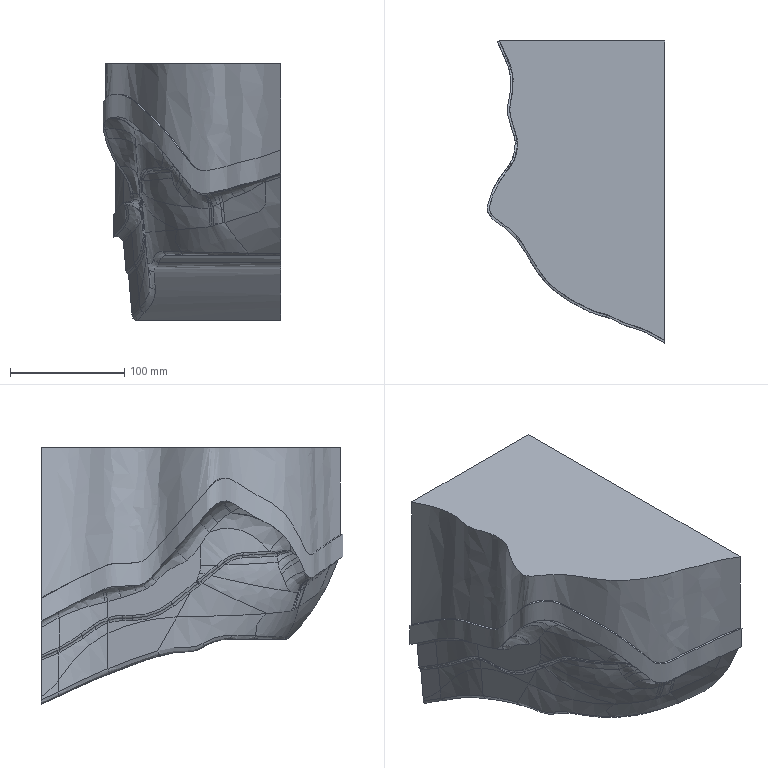Part | NX | features solid 2 | 1 solid | 122 faces | box 155.829 x 264.379 x 224.846 mm | volume 5315383 mm3 | spline 117 | plane 4 | cylinder 1 | commonest cylinder face diameters 80 x1